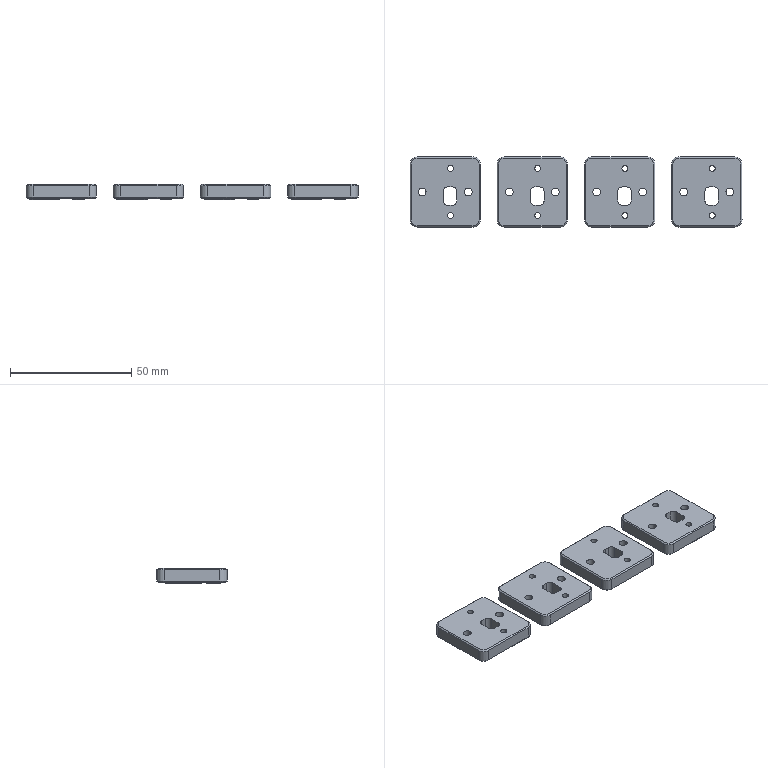NC program | NX | posted with a generic post | part box 137 x 29 x 6.3 mm
Lines 3358 to 3650 of 3650:
(ZLEVEL_PROFILE_1_COPY_1_COPY_COPY_COPY , TOOL : D4A45)
N6708 T02 M6
N6710 G54
N6712 G17 G0 G90 X20.2 Y-9.991 S9500 M3
N6714 G43 Z30. H2
N6716 Z0.43
N6718 G94 G1 Z-1.57 F1000.
N6720 G3 X20.491 Y-9.7 R0.291
N6722 X20.2 Y-9.991 R-0.291
N6724 X20.373 Y-9.891 R0.2
N6726 G1 Z-0.57
N6728 G0 Z30.
N6730 X20.2 Y9.991
N6732 Z0.43
N6734 G1 Z-1.57
N6736 G3 X19.909 Y9.7 R0.291
N6738 X20.2 Y9.991 R-0.291
N6740 X20.027 Y9.891 R0.2
N6742 G1 Z-0.57
N6744 G0 Z30.
N6746 X8.717 Y0.043
N6748 Z0.43
N6750 G1 Z-1.57
N6752 G2 X8.695 Y0.663 R1.929
N6754 G3 X7.885 Y-0.316 R0.691
N6756 G2 X8.498 Y-0.221 R1.929
N6758 G3 X8.717 Y0.043 R0.221
N6760 X8.453 Y0.344 R0.4
N6762 G1 Z-0.57
N6764 G0 Z30.
N6766 X27.5 Y0.691
N6768 Z0.43
N6770 G1 Z-1.57
N6772 G3 X26.809 Y0. R0.691
N6774 X27.5 Y0.691 R-0.691
N6776 X27.154 Y0.491 R0.4
N6778 G1 Z-0.57
N6780 G0 Z30.
N6782 X21.036 Y-0.293
N6784 Z-0.57
N6786 G1 Z-1.57
N6788 X21.641 Y-0.619
N6790 G3 X21.841 Y-0.273 R0.4
N6792 G1 Y3.727
N6794 G3 X21. Y4.569 R0.841
N6796 G1 X19.
N6798 G3 X18.337 Y4.246 R0.841
N6800 G2 X18.628 Y3.245 R1.929
N6802 G1 Y1.076
N6804 G2 X18.158 Y-0.176 R1.929
N6806 G1 Y-0.273
N6808 G3 X19. Y-1.114 R0.841
N6810 G1 X21.
N6812 G3 X21.841 Y-0.273 R0.841
N6814 X21.641 Y0.074 R0.4
N6816 G1 X21.041 Y0.42
N6818 Z-0.57
N6820 G0 Z30.
N6822 X56.2 Y-9.991
N6824 Z0.43
N6826 G1 Z-1.57
N6828 G3 X56.491 Y-9.7 R0.291
N6830 X56.2 Y-9.991 R-0.291
N6832 X56.373 Y-9.891 R0.2
N6834 G1 Z-0.57
N6836 G0 Z30.
N6838 X56.2 Y9.991
N6840 Z0.43
N6842 G1 Z-1.57
N6844 G3 X55.909 Y9.7 R0.291
N6846 X56.2 Y9.991 R-0.291
N6848 X56.027 Y9.891 R0.2
N6850 G1 Z-0.57
N6852 G0 Z30.
N6854 X64.191 Y0.
N6856 Z0.43
N6858 G1 Z-1.57
N6860 Y0.001
N6862 G3 X63.499 Y0.691 R0.691
N6864 X64.191 Y0. R-0.691
N6866 X63.991 Y0.346 R0.4
N6868 G1 Z-0.57
N6870 G0 Z30.
N6872 X44.717 Y0.043
N6874 Z0.43
N6876 G1 Z-1.57
N6878 G2 X44.695 Y0.663 R1.929
N6880 G3 X43.885 Y-0.316 R0.691
N6882 G2 X44.498 Y-0.221 R1.929
N6884 G3 X44.717 Y0.043 R0.221
N6886 X44.453 Y0.344 R0.4
N6888 G1 Z-0.57
N6890 G0 Z30.
N6892 X57.036 Y-0.293
N6894 Z-0.57
N6896 G1 Z-1.57
N6898 X57.641 Y-0.619
N6900 G3 X57.841 Y-0.273 R0.4
N6902 G1 Y3.727
N6904 G3 X57. Y4.569 R0.841
N6906 G1 X55.
N6908 G3 X54.337 Y4.246 R0.841
N6910 G2 X54.628 Y3.245 R1.929
N6912 G1 Y1.076
N6914 G2 X54.158 Y-0.176 R1.929
N6916 G1 Y-0.273
N6918 G3 X55. Y-1.114 R0.841
N6920 G1 X57.
N6922 G3 X57.841 Y-0.273 R0.841
N6924 X57.641 Y0.074 R0.4
N6926 G1 X57.041 Y0.42
N6928 Z-0.57
N6930 G0 Z30.
N6932 X-51.8 Y9.991
N6934 Z0.43
N6936 G1 Z-1.57
N6938 G3 X-52.091 Y9.7 R0.291
N6940 X-51.8 Y9.991 R-0.291
N6942 X-51.973 Y9.891 R0.2
N6944 G1 Z-0.57
N6946 G0 Z30.
N6948 X-44.5 Y0.691
N6950 Z0.43
N6952 G1 Z-1.57
N6954 G3 X-45.191 Y0. R0.691
N6956 X-44.5 Y0.691 R-0.691
N6958 X-44.846 Y0.491 R0.4
N6960 G1 Z-0.57
N6962 G0 Z30.
N6964 X-63.283 Y0.043
N6966 Z0.43
N6968 G1 Z-1.57
N6970 G2 X-63.305 Y0.663 R1.929
N6972 G3 X-64.115 Y-0.316 R0.691
N6974 G2 X-63.502 Y-0.221 R1.929
N6976 G3 X-63.283 Y0.043 R0.221
N6978 X-63.547 Y0.344 R0.4
N6980 G1 Z-0.57
N6982 G0 Z30.
N6984 X-50.964 Y-0.293
N6986 Z-0.57
N6988 G1 Z-1.57
N6990 X-50.359 Y-0.619
N6992 G3 X-50.159 Y-0.273 R0.4
N6994 G1 Y3.727
N6996 G3 X-51. Y4.569 R0.841
N6998 G1 X-53.
N7000 G3 X-53.663 Y4.246 R0.841
N7002 G2 X-53.372 Y3.245 R1.929
N7004 G1 Y1.076
N7006 G2 X-53.842 Y-0.176 R1.929
N7008 G1 Y-0.273
N7010 G3 X-53. Y-1.114 R0.841
N7012 G1 X-51.
N7014 G3 X-50.159 Y-0.273 R0.841
N7016 X-50.359 Y0.074 R0.4
N7018 G1 X-50.959 Y0.42
N7020 Z-0.57
N7022 G0 Z30.
N7024 X-51.8 Y-9.991
N7026 Z0.43
N7028 G1 Z-1.57
N7030 G3 X-51.509 Y-9.7 R0.291
N7032 X-51.8 Y-9.991 R-0.291
N7034 X-51.627 Y-9.891 R0.2
N7036 G1 Z-0.57
N7038 G0 Z30.
N7040 X-15.8 Y9.991
N7042 Z0.43
N7044 G1 Z-1.57
N7046 G3 X-16.091 Y9.7 R0.291
N7048 X-15.8 Y9.991 R-0.291
N7050 X-15.973 Y9.891 R0.2
N7052 G1 Z-0.57
N7054 G0 Z30.
N7056 X-8.5 Y0.691
N7058 Z0.43
N7060 G1 Z-1.57
N7062 G3 X-9.191 Y0. R0.691
N7064 X-8.5 Y0.691 R-0.691
N7066 X-8.846 Y0.491 R0.4
N7068 G1 Z-0.57
N7070 G0 Z30.
N7072 X-27.283 Y0.043
N7074 Z0.43
N7076 G1 Z-1.57
N7078 G2 X-27.305 Y0.663 R1.929
N7080 G3 X-28.115 Y-0.316 R0.691
N7082 G2 X-27.502 Y-0.221 R1.929
N7084 G3 X-27.283 Y0.043 R0.221
N7086 X-27.547 Y0.344 R0.4
N7088 G1 Z-0.57
N7090 G0 Z30.
N7092 X-14.964 Y-0.293
N7094 Z-0.57
N7096 G1 Z-1.57
N7098 X-14.359 Y-0.619
N7100 G3 X-14.159 Y-0.273 R0.4
N7102 G1 Y3.727
N7104 G3 X-15. Y4.569 R0.841
N7106 G1 X-17.
N7108 G3 X-17.663 Y4.246 R0.841
N7110 G2 X-17.372 Y3.241 R1.929
N7112 G1 Y1.081
N7114 G2 X-17.842 Y-0.176 R1.929
N7116 G1 Y-0.273
N7118 G3 X-17. Y-1.114 R0.841
N7120 G1 X-15.
N7122 G3 X-14.159 Y-0.273 R0.841
N7124 X-14.359 Y0.074 R0.4
N7126 G1 X-14.959 Y0.42
N7128 Z-0.57
N7130 G0 Z30.
N7132 X-15.8 Y-9.991
N7134 Z0.43
N7136 G1 Z-1.57
N7138 G3 X-15.509 Y-9.7 R0.291
N7140 X-15.8 Y-9.991 R-0.291
N7142 X-15.627 Y-9.891 R0.2
N7144 G1 Z-0.57
N7146 G0 Z30.
N7148 X-5.837 Y-15.707
N7150 Z-0.57
N7152 G1 Z-1.57
N7154 X-6.154 Y-15.159
N7156 G3 X-6.5 Y-14.959 R0.4
N7158 G1 X-29.502
N7160 G2 X-32.959 Y-11.5 R3.459
N7162 G1 Y11.503
N7164 G2 X-29.5 Y14.959 R3.459
N7166 G1 X-6.497
N7168 G2 X-3.041 Y11.5 R3.459
N7170 G1 Y-11.502
N7172 G2 X-6.5 Y-14.959 R3.459
N7174 G3 X-6.846 Y-15.159 R0.4
N7176 G1 X-7.193 Y-15.759
N7178 Z-0.57
N7180 G0 Z30.
N7182 X-41.837 Y-15.707
N7184 Z-0.57
N7186 G1 Z-1.57
N7188 X-42.154 Y-15.159
N7190 G3 X-42.5 Y-14.959 R0.4
N7192 G1 X-65.502
N7194 G2 X-68.959 Y-11.5 R3.459
N7196 G1 Y11.502
N7198 G2 X-65.5 Y14.959 R3.459
N7200 G1 X-42.497
N7202 G2 X-39.041 Y11.5 R3.459
N7204 G1 Y-11.502
N7206 G2 X-42.5 Y-14.959 R3.459
N7208 G3 X-42.846 Y-15.159 R0.4
N7210 G1 X-43.193 Y-15.759
N7212 Z-0.57
N7214 G0 Z30.
N7216 X66.163 Y-15.707
N7218 Z-0.57
N7220 G1 Z-1.57
N7222 X65.846 Y-15.159
N7224 G3 X65.5 Y-14.959 R0.4
N7226 G1 X42.497
N7228 G2 X39.041 Y-11.5 R3.459
N7230 G1 Y11.502
N7232 G2 X42.5 Y14.959 R3.459
N7234 G1 X65.502
N7236 G2 X68.959 Y11.5 R3.459
N7238 G1 Y-11.502
N7240 G2 X65.5 Y-14.959 R3.459
N7242 G3 X65.154 Y-15.159 R0.4
N7244 G1 X64.807 Y-15.759
N7246 Z-0.57
N7248 G0 Z30.
N7250 X30.163 Y-15.707
N7252 Z-0.57
N7254 G1 Z-1.57
N7256 X29.846 Y-15.159
N7258 G3 X29.5 Y-14.959 R0.4
N7260 G1 X6.497
N7262 G2 X3.041 Y-11.5 R3.459
N7264 G1 Y11.502
N7266 G2 X6.5 Y14.959 R3.459
N7268 G1 X29.502
N7270 G2 X32.959 Y11.5 R3.459
N7272 G1 Y-11.503
N7274 G2 X29.5 Y-14.959 R3.459
N7276 G3 X29.154 Y-15.159 R0.4
N7278 G1 X28.807 Y-15.759
N7280 Z-0.57
N7282 G0 Z30.
N7284 M5
N7286 M2